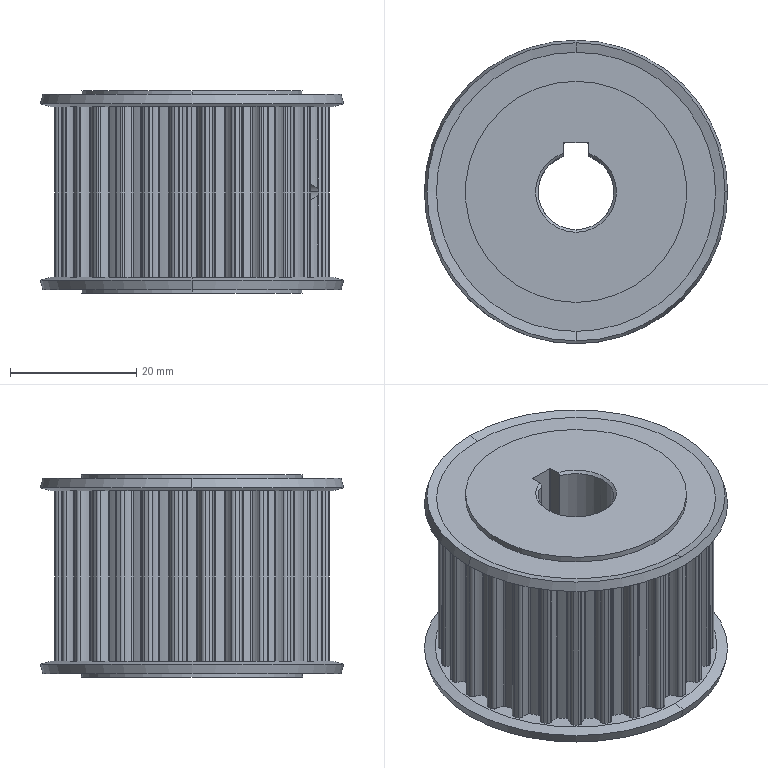Part | SolidWorks | features BaseBody 1 | 1 solid | 300 faces | box 48 x 48 x 32 mm | volume 40101 mm3 | cylinder 274 | cone 17 | plane 9 | commonest cylinder face diameters 0.5 x70 1.1 x69 6.55 x64 40.06 x31 43.6 x28 3.242 x4